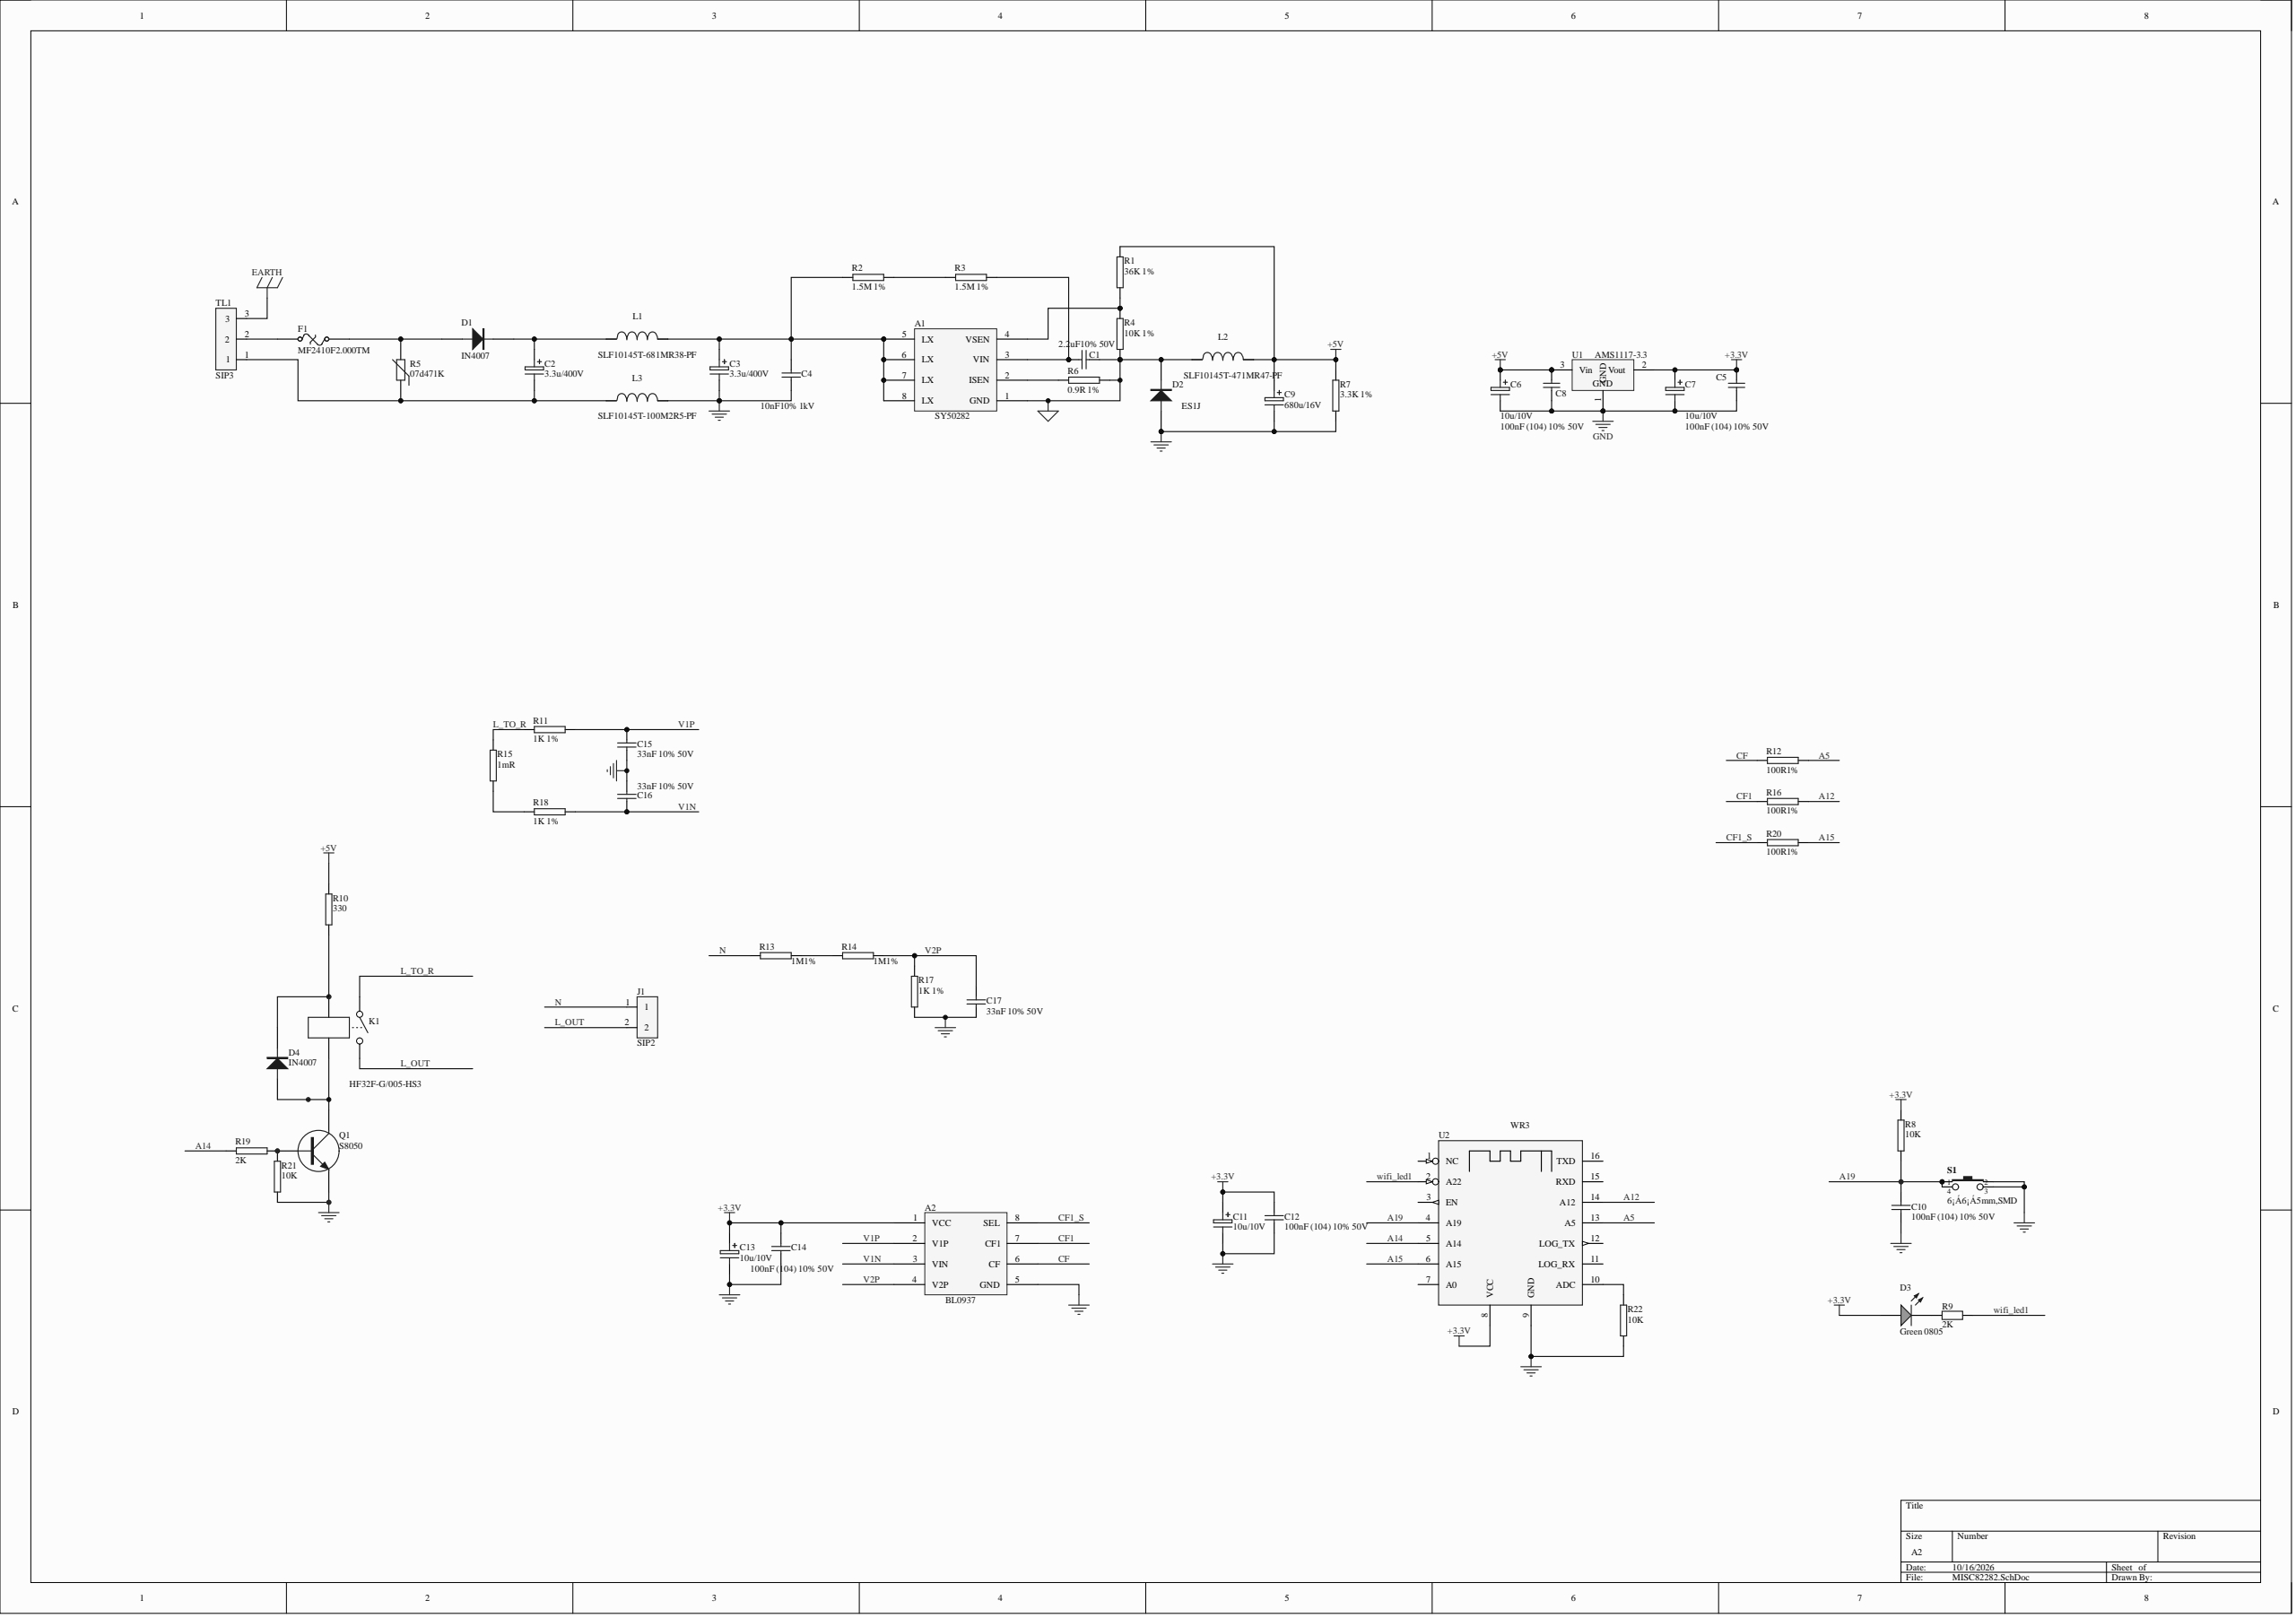Circuit board | Altium Designer | 56 parts | 35 nets
Bill of materials:
Comment,Description,Designator,Footprint,LibRef,Quantity
"SY50282","","A1","SO-8","TPS54331DR","1"
"BL0937","","A2","SO-8","TPS54331DR","1"
"2.2uF10% 50V","Capacitor","C1","0603","CAP","1"
"3.3u/400V","","C2, C3","SMD8x10.5","ELECTRO1","2"
"10nF10% 1kV","Capacitor","C4","1206","CAP","1"
"100nF (104) 10% 50V","SMD capacitor, Capacitor","C5, C8, C10, C12, C14","0603","0603 100nF (104) 10% 50V, CAP","5"
"10u/10V","","C6, C7, C11, C13","0805","ELECTRO1","4"
"680u/16V","","C9","10X12.5","ELECTRO1","1"
"33nF 10% 50V","Capacitor","C15, C16, C17","0603","CAP","3"
"IN4007","Diode","D1, D4","SDIODE-2","DIODE","2"
"ES1J","Diode","D2","SDIODE-2","DIODE","1"
"Green 0805","LED","D3","0805_LED_S1","0805 翠绿","1"
"MF2410F2.000TM","Thermal Fuse","F1","2410","Fuse Thermal","1"
"SIP2","","J1","DIP-2","SIP2","1"
"HF32F-G/005-HS3","","K1","HF32F-G/005-HS3","RELAY-SPST","1"
"VLP8040T-3R3N","Unknown","L1, L2, L3","IND10X10","VLP8040T-3R3N","3"
"S8050","","Q1","SOT-23(SOT-23-3)","NPN-1","1"
"36K 1%","","R1","1206","RES2","1"
"1.5M 1%","","R2, R3","1206","RES2","2"
"10K 1%","","R4","0805","RES2","1"
"07d471K","Varistor (Voltage-Sensitive Resistor)","R5","07d471K","Res Varistor","1"
"0.9R 1%","","R6","0805","RES2","1"
"3.3K 1%","","R7","0805","RES2","1"
"10K","","R8, R21, R22","0603","RES2","3"
"2K","SMD resistor, [NoValue]","R9, R19","0603","0603 680|¸ (6800) 1%, RES2","2"
"330","","R10","1206","RES2","1"
"1K 1%","","R11, R17, R18","0603","RES2","3"
"100R1%","","R12, R16, R20","0603","RES2","3"
"1M1%","","R13, R14","1206","RES2","2"
"1mR","","R15","2512","RES2","1"
"SW-PB4P","6¡Á6¡Á5.0mm, black, SMD,,*","S1","smd6X6x4.5","","1"
"SIP3","","TL1","DIP-3","SIP3","1"
"AMS1117-3.3","Low-dropout linear regulator (LDO)","U1","SOT-223","SOT-223 AMS1117-3.3","1"
"WR3","","U2","WR3","SR_FRS_1WV","1"
Netlist (Protel format):
[
A1
SO-8
SY50282



]
[
A2
SO-8
BL0937



]
[
C1
0603
2.2uF10% 50V



]
[
C2
SMD8x10.5
3.3u/400V



]
[
C3
SMD8x10.5
3.3u/400V



]
[
C4
1206
10nF10% 1kV



]
[
C5
0603
100nF (104) 10% 50V



]
[
C6
0805
10u/10V



]
[
C7
0805
10u/10V



]
[
C8
0603
100nF (104) 10% 50V



]
[
C9
10X12.5
680u/16V



]
[
C10
0603
100nF (104) 10% 50V



]
[
C11
0805
10u/10V



]
[
C12
0603
100nF (104) 10% 50V



]
[
C13
0805
10u/10V



]
[
C14
0603
100nF (104) 10% 50V



]
[
C15
0603
33nF 10% 50V



]
[
C16
0603
33nF 10% 50V



]
[
C17
0603
33nF 10% 50V



]
[
D1
SDIODE-2
IN4007



]
[
D2
SDIODE-2
ES1J



]
[
D3
0805_LED_S1
Green 0805



]
[
D4
SDIODE-2
IN4007



]
[
F1
2410
MF2410F2.000TM



]
[
J1
DIP-2
SIP2



]
[
K1
HF32F-G/005-HS3
HF32F-G/005-HS3



]
[
L1
IND10X10
VLP8040T-3R3N



]
[
L2
IND10X10
VLP8040T-3R3N



]
[
L3
IND10X10
VLP8040T-3R3N



]
[
Q1
SOT-23(SOT-23-3)
S8050



]
[
R1
1206
36K 1%



]
[
R2
1206
1.5M 1%



]
[
R3
1206
1.5M 1%



]
[
R4
0805
10K 1%



]
[
R5
07d471K
07d471K



]
[
R6
0805
0.9R 1%



]
[
R7
0805
3.3K 1%



]
[
R8
0603
10K



]
[
R9
0603
2K



]
[
R10
1206
330



]
[
R11
0603
1K 1%



]
[
R12
0603
100R1%



]
[
R13
1206
1M1%



]
[
R14
1206
1M1%



]
[
R15
2512
1mR



]
[
R16
0603
100R1%



]
[
R17
0603
1K 1%



]
[
R18
0603
1K 1%



]
[
R19
0603
2K



]
[
R20
0603
100R1%



]
[
R21
0603
10K



]
[
R22
0603
10K



]
[
S1
smd6X6x4.5
SW-PB4P



]
[
TL1
DIP-3
SIP3



]
[
U1
SOT-223
AMS1117-3.3



]
[
U2
WR3
WR3



]
(
wifi_led1
R9-1
U2-2
)
(
V2P
A2-4
C17-1
R14-2
R17-1
)
(
V1P
A2-2
C15-1
R11-1
)
(
V1N
A2-3
C16-2
R18-1
)
(
NetR22_1
R22-1
U2-10
)
(
NetR15_2
R15-2
R18-2
)
(
NetR13_2
R13-2
R14-1
)
(
NetR2_2
R2-2
R3-1
)
(
NetQ1_1
Q1-1
R19-1
R21-1
)
(
NetF1_1
F1-1
TL1-2
)
(
NetD4_K
D4-K
K1-1
R10-1
)
(
NetD4_A
D4-A
K1-2
Q1-3
)
(
NetD3_K
D3-K
R9-2
)
(
NetD1_A
D1-A
F1-2
R5-2
)
(
NetC2_2
C2-2
L3-2
R5-1
TL1-1
)
(
NetC2_1
C2-1
D1-K
L1-2
)
(
NetA1_5
A1-5
A1-6
A1-7
A1-8
C3-1
C4-1
L1-1
R2-1
)
(
NetA1_4
A1-4
R1-2
R4-1
)
(
NetA1_3
A1-3
C1-1
R3-2
)
(
NetA1_2
A1-2
R6-1
)
(
N
J1-1
R13-1
)
(
L_TO_R
K1-3
R11-2
R15-1
)
(
L_OUT
J1-2
K1-4
)
(
GNDS
A1-1
C1-2
D2-K
L2-2
R4-2
R6-2
)
(
GND
A2-5
C3-2
C4-2
C5-2
C6-2
C7-2
C8-2
C9-2
C10-2
C11-2
C12-2
C13-2
C14-2
C15-2
C16-1
C17-2
D2-A
L3-1
Q1-2
R7-2
R17-2
R21-2
R22-2
S1-2
S1-3
U1-1
U2-9
)
(
CF1_S
A2-8
R20-1
)
(
CF1
A2-7
R16-1
)
(
CF
A2-6
R12-1
)
(
A19
C10-1
R8-2
S1-1
S1-4
U2-4
)
(
A15
R20-2
U2-6
)
(
A14
R19-2
U2-5
)
(
A12
R16-2
U2-14
)
(
A5
R12-2
U2-13
)
(
+5V
C6-1
C8-1
C9-1
L2-1
R1-1
R7-1
R10-2
U1-3
)
(
+3.3V
A2-1
C5-1
C7-1
C11-1
C12-1
C13-1
C14-1
D3-A
R8-1
U1-2
U2-8
)